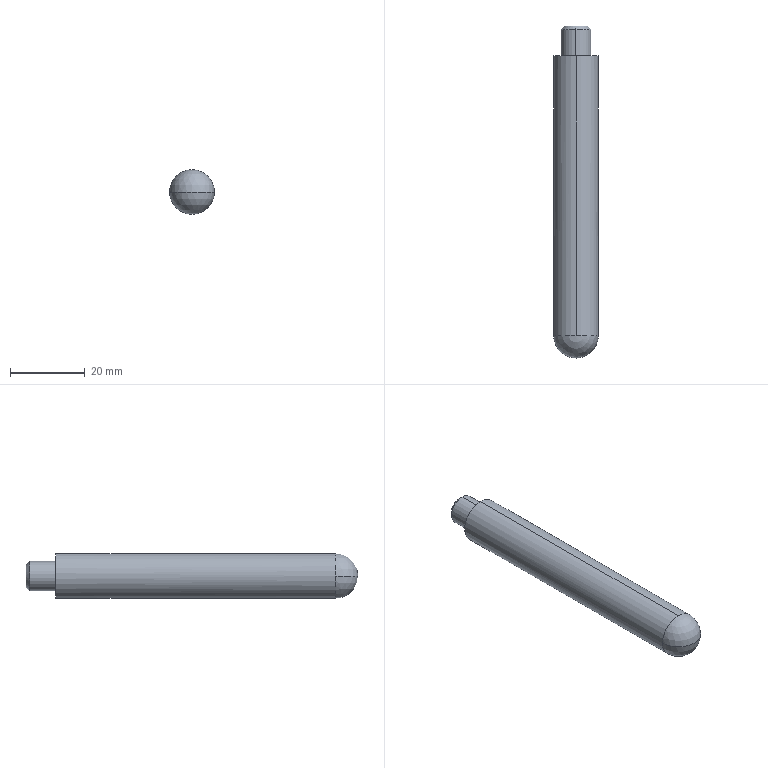Part | SolidWorks | features Chamfer 1, Revolution 1 | 1 solid | 10 faces | box 12 x 89 x 12 mm | volume 9325 mm3 | cylinder 4 | cone 2 | sphere 2 | plane 2 | commonest cylinder face diameters 8 x2 12 x2
STEP:
#1=CARTESIAN_POINT('',(0.,90.,3.));
#2=VERTEX_POINT('',#1);
#3=CARTESIAN_POINT('',(0.,90.,-3.));
#4=VERTEX_POINT('',#3);
#5=CARTESIAN_POINT('',(0.,90.,0.));
#6=DIRECTION('',(0.,1.,0.));
#7=DIRECTION('',(0.,0.,-1.));
#8=AXIS2_PLACEMENT_3D('',#5,#6,#7);
#9=CIRCLE('',#8,3.);
#10=EDGE_CURVE('',#2,#4,#9,.T.);
#11=ORIENTED_EDGE('',*,*,#10,.F.);
#12=CARTESIAN_POINT('',(0.,89.,4.));
#13=VERTEX_POINT('',#12);
#14=CARTESIAN_POINT('',(0.,89.,4.));
#15=DIRECTION('',(0.,-0.7071,0.7071));
#16=VECTOR('',#15,1000.);
#17=LINE('',#14,#16);
#18=EDGE_CURVE('',#2,#13,#17,.T.);
#19=ORIENTED_EDGE('',*,*,#18,.T.);
#20=CARTESIAN_POINT('',(0.,89.,-4.));
#21=VERTEX_POINT('',#20);
#22=CARTESIAN_POINT('',(0.,89.,0.));
#23=DIRECTION('',(0.,-1.,0.));
#24=DIRECTION('',(0.,0.,-1.));
#25=AXIS2_PLACEMENT_3D('',#22,#23,#24);
#26=CIRCLE('',#25,4.);
#27=EDGE_CURVE('',#21,#13,#26,.T.);
#28=ORIENTED_EDGE('',*,*,#27,.F.);
#29=CARTESIAN_POINT('',(0.,89.,-4.));
#30=DIRECTION('',(0.,-0.7071,-0.7071));
#31=VECTOR('',#30,1000.);
#32=LINE('',#29,#31);
#33=EDGE_CURVE('',#4,#21,#32,.T.);
#34=ORIENTED_EDGE('',*,*,#33,.F.);
#35=EDGE_LOOP('',(#11,#19,#28,#34));
#36=FACE_OUTER_BOUND('',#35,.T.);
#37=CARTESIAN_POINT('',(0.,89.,0.));
#38=DIRECTION('',(0.,-1.,0.));
#39=DIRECTION('',(0.,0.,-1.));
#40=AXIS2_PLACEMENT_3D('',#37,#38,#39);
#41=CONICAL_SURFACE('',#40,4.,0.7854);
#42=ADVANCED_FACE('',(#36),#41,.T.);
#43=CARTESIAN_POINT('',(0.,7.,-6.));
#44=VERTEX_POINT('',#43);
#45=CARTESIAN_POINT('',(6.,7.,0.));
#46=VERTEX_POINT('',#45);
#47=CARTESIAN_POINT('',(0.,7.,0.));
#48=DIRECTION('',(0.,-1.,0.));
#49=DIRECTION('',(0.,0.,-1.));
#50=AXIS2_PLACEMENT_3D('',#47,#48,#49);
#51=CIRCLE('',#50,6.);
#52=EDGE_CURVE('',#44,#46,#51,.T.);
#53=ORIENTED_EDGE('',*,*,#52,.T.);
#54=CARTESIAN_POINT('',(0.,1.,0.));
#55=VERTEX_POINT('',#54);
#56=CARTESIAN_POINT('',(0.,7.,0.));
#57=DIRECTION('',(0.,0.,-1.));
#58=DIRECTION('',(-1.,0.,0.));
#59=AXIS2_PLACEMENT_3D('',#56,#57,#58);
#60=CIRCLE('',#59,6.);
#61=EDGE_CURVE('',#46,#55,#60,.T.);
#62=ORIENTED_EDGE('',*,*,#61,.T.);
#63=CARTESIAN_POINT('',(-6.,7.,0.));
#64=VERTEX_POINT('',#63);
#65=CARTESIAN_POINT('',(0.,7.,0.));
#66=DIRECTION('',(0.,0.,1.));
#67=DIRECTION('',(1.,0.,0.));
#68=AXIS2_PLACEMENT_3D('',#65,#66,#67);
#69=CIRCLE('',#68,6.);
#70=EDGE_CURVE('',#64,#55,#69,.T.);
#71=ORIENTED_EDGE('',*,*,#70,.F.);
#72=CARTESIAN_POINT('',(0.,7.,0.));
#73=DIRECTION('',(0.,-1.,0.));
#74=DIRECTION('',(0.,0.,-1.));
#75=AXIS2_PLACEMENT_3D('',#72,#73,#74);
#76=CIRCLE('',#75,6.);
#77=EDGE_CURVE('',#64,#44,#76,.T.);
#78=ORIENTED_EDGE('',*,*,#77,.T.);
#79=EDGE_LOOP('',(#53,#62,#71,#78));
#80=FACE_OUTER_BOUND('',#79,.T.);
#81=CARTESIAN_POINT('',(0.,7.,0.));
#82=DIRECTION('',(0.,0.,-1.));
#83=DIRECTION('',(-1.,0.,0.));
#84=AXIS2_PLACEMENT_3D('',#81,#82,#83);
#85=SPHERICAL_SURFACE('',#84,6.);
#86=ADVANCED_FACE('',(#80),#85,.T.);
#87=CARTESIAN_POINT('',(0.,82.,-6.));
#88=VERTEX_POINT('',#87);
#89=CARTESIAN_POINT('',(0.,82.,6.));
#90=VERTEX_POINT('',#89);
#91=CARTESIAN_POINT('',(0.,82.,0.));
#92=DIRECTION('',(0.,-1.,0.));
#93=DIRECTION('',(0.,0.,-1.));
#94=AXIS2_PLACEMENT_3D('',#91,#92,#93);
#95=CIRCLE('',#94,6.);
#96=EDGE_CURVE('',#88,#90,#95,.T.);
#97=ORIENTED_EDGE('',*,*,#96,.T.);
#98=CARTESIAN_POINT('',(0.,7.,6.));
#99=VERTEX_POINT('',#98);
#100=CARTESIAN_POINT('',(0.,0.,6.));
#101=DIRECTION('',(0.,-1.,0.));
#102=VECTOR('',#101,1000.);
#103=LINE('',#100,#102);
#104=EDGE_CURVE('',#90,#99,#103,.T.);
#105=ORIENTED_EDGE('',*,*,#104,.T.);
#106=CARTESIAN_POINT('',(0.,7.,0.));
#107=DIRECTION('',(0.,-1.,0.));
#108=DIRECTION('',(0.,0.,-1.));
#109=AXIS2_PLACEMENT_3D('',#106,#107,#108);
#110=CIRCLE('',#109,6.);
#111=EDGE_CURVE('',#46,#99,#110,.T.);
#112=ORIENTED_EDGE('',*,*,#111,.F.);
#113=ORIENTED_EDGE('',*,*,#52,.F.);
#114=CARTESIAN_POINT('',(0.,0.,-6.));
#115=DIRECTION('',(0.,-1.,0.));
#116=VECTOR('',#115,1000.);
#117=LINE('',#114,#116);
#118=EDGE_CURVE('',#88,#44,#117,.T.);
#119=ORIENTED_EDGE('',*,*,#118,.F.);
#120=EDGE_LOOP('',(#97,#105,#112,#113,#119));
#121=FACE_OUTER_BOUND('',#120,.T.);
#122=CARTESIAN_POINT('',(0.,0.,0.));
#123=DIRECTION('',(0.,-1.,0.));
#124=DIRECTION('',(0.,0.,-1.));
#125=AXIS2_PLACEMENT_3D('',#122,#123,#124);
#126=CYLINDRICAL_SURFACE('',#125,6.);
#127=ADVANCED_FACE('',(#121),#126,.T.);
#128=ORIENTED_EDGE('',*,*,#27,.T.);
#129=CARTESIAN_POINT('',(0.,82.,4.));
#130=VERTEX_POINT('',#129);
#131=CARTESIAN_POINT('',(0.,0.,4.));
#132=DIRECTION('',(0.,-1.,0.));
#133=VECTOR('',#132,1000.);
#134=LINE('',#131,#133);
#135=EDGE_CURVE('',#13,#130,#134,.T.);
#136=ORIENTED_EDGE('',*,*,#135,.T.);
#137=CARTESIAN_POINT('',(0.,82.,-4.));
#138=VERTEX_POINT('',#137);
#139=CARTESIAN_POINT('',(0.,82.,0.));
#140=DIRECTION('',(0.,-1.,0.));
#141=DIRECTION('',(0.,0.,-1.));
#142=AXIS2_PLACEMENT_3D('',#139,#140,#141);
#143=CIRCLE('',#142,4.);
#144=EDGE_CURVE('',#138,#130,#143,.T.);
#145=ORIENTED_EDGE('',*,*,#144,.F.);
#146=CARTESIAN_POINT('',(0.,0.,-4.));
#147=DIRECTION('',(0.,-1.,0.));
#148=VECTOR('',#147,1000.);
#149=LINE('',#146,#148);
#150=EDGE_CURVE('',#21,#138,#149,.T.);
#151=ORIENTED_EDGE('',*,*,#150,.F.);
#152=EDGE_LOOP('',(#128,#136,#145,#151));
#153=FACE_OUTER_BOUND('',#152,.T.);
#154=CARTESIAN_POINT('',(0.,0.,0.));
#155=DIRECTION('',(0.,-1.,0.));
#156=DIRECTION('',(0.,0.,-1.));
#157=AXIS2_PLACEMENT_3D('',#154,#155,#156);
#158=CYLINDRICAL_SURFACE('',#157,4.);
#159=ADVANCED_FACE('',(#153),#158,.T.);
#160=CARTESIAN_POINT('',(0.,90.,0.));
#161=DIRECTION('',(0.,1.,0.));
#162=DIRECTION('',(0.,0.,-1.));
#163=AXIS2_PLACEMENT_3D('',#160,#161,#162);
#164=CIRCLE('',#163,3.);
#165=EDGE_CURVE('',#4,#2,#164,.T.);
#166=ORIENTED_EDGE('',*,*,#165,.T.);
#167=ORIENTED_EDGE('',*,*,#10,.T.);
#168=EDGE_LOOP('',(#166,#167));
#169=FACE_OUTER_BOUND('',#168,.T.);
#170=CARTESIAN_POINT('',(0.,90.,0.));
#171=DIRECTION('',(0.,-1.,0.));
#172=DIRECTION('',(0.,0.,-1.));
#173=AXIS2_PLACEMENT_3D('',#170,#171,#172);
#174=PLANE('',#173);
#175=ADVANCED_FACE('',(#169),#174,.F.);
#176=ORIENTED_EDGE('',*,*,#135,.F.);
#177=CARTESIAN_POINT('',(0.,89.,0.));
#178=DIRECTION('',(0.,-1.,0.));
#179=DIRECTION('',(0.,0.,-1.));
#180=AXIS2_PLACEMENT_3D('',#177,#178,#179);
#181=CIRCLE('',#180,4.);
#182=EDGE_CURVE('',#13,#21,#181,.T.);
#183=ORIENTED_EDGE('',*,*,#182,.T.);
#184=ORIENTED_EDGE('',*,*,#150,.T.);
#185=CARTESIAN_POINT('',(0.,82.,0.));
#186=DIRECTION('',(0.,-1.,0.));
#187=DIRECTION('',(0.,0.,-1.));
#188=AXIS2_PLACEMENT_3D('',#185,#186,#187);
#189=CIRCLE('',#188,4.);
#190=EDGE_CURVE('',#130,#138,#189,.T.);
#191=ORIENTED_EDGE('',*,*,#190,.F.);
#192=EDGE_LOOP('',(#176,#183,#184,#191));
#193=FACE_OUTER_BOUND('',#192,.T.);
#194=CARTESIAN_POINT('',(0.,0.,0.));
#195=DIRECTION('',(0.,-1.,0.));
#196=DIRECTION('',(0.,0.,-1.));
#197=AXIS2_PLACEMENT_3D('',#194,#195,#196);
#198=CYLINDRICAL_SURFACE('',#197,4.);
#199=ADVANCED_FACE('',(#193),#198,.T.);
#200=ORIENTED_EDGE('',*,*,#96,.F.);
#201=CARTESIAN_POINT('',(0.,82.,0.));
#202=DIRECTION('',(0.,-1.,0.));
#203=DIRECTION('',(0.,0.,-1.));
#204=AXIS2_PLACEMENT_3D('',#201,#202,#203);
#205=CIRCLE('',#204,6.);
#206=EDGE_CURVE('',#90,#88,#205,.T.);
#207=ORIENTED_EDGE('',*,*,#206,.F.);
#208=EDGE_LOOP('',(#200,#207));
#209=FACE_OUTER_BOUND('',#208,.T.);
#210=ORIENTED_EDGE('',*,*,#144,.T.);
#211=ORIENTED_EDGE('',*,*,#190,.T.);
#212=EDGE_LOOP('',(#210,#211));
#213=FACE_BOUND('',#212,.T.);
#214=CARTESIAN_POINT('',(-4.,82.,0.));
#215=DIRECTION('',(0.,-1.,0.));
#216=DIRECTION('',(0.,0.,-1.));
#217=AXIS2_PLACEMENT_3D('',#214,#215,#216);
#218=PLANE('',#217);
#219=ADVANCED_FACE('',(#209,#213),#218,.F.);
#220=ORIENTED_EDGE('',*,*,#104,.F.);
#221=ORIENTED_EDGE('',*,*,#206,.T.);
#222=ORIENTED_EDGE('',*,*,#118,.T.);
#223=ORIENTED_EDGE('',*,*,#77,.F.);
#224=CARTESIAN_POINT('',(0.,7.,0.));
#225=DIRECTION('',(0.,-1.,0.));
#226=DIRECTION('',(0.,0.,-1.));
#227=AXIS2_PLACEMENT_3D('',#224,#225,#226);
#228=CIRCLE('',#227,6.);
#229=EDGE_CURVE('',#99,#64,#228,.T.);
#230=ORIENTED_EDGE('',*,*,#229,.F.);
#231=EDGE_LOOP('',(#220,#221,#222,#223,#230));
#232=FACE_OUTER_BOUND('',#231,.T.);
#233=CARTESIAN_POINT('',(0.,0.,0.));
#234=DIRECTION('',(0.,-1.,0.));
#235=DIRECTION('',(0.,0.,-1.));
#236=AXIS2_PLACEMENT_3D('',#233,#234,#235);
#237=CYLINDRICAL_SURFACE('',#236,6.);
#238=ADVANCED_FACE('',(#232),#237,.T.);
#239=ORIENTED_EDGE('',*,*,#61,.F.);
#240=ORIENTED_EDGE('',*,*,#111,.T.);
#241=ORIENTED_EDGE('',*,*,#229,.T.);
#242=ORIENTED_EDGE('',*,*,#70,.T.);
#243=EDGE_LOOP('',(#239,#240,#241,#242));
#244=FACE_OUTER_BOUND('',#243,.T.);
#245=CARTESIAN_POINT('',(0.,7.,0.));
#246=DIRECTION('',(0.,0.,-1.));
#247=DIRECTION('',(-1.,0.,0.));
#248=AXIS2_PLACEMENT_3D('',#245,#246,#247);
#249=SPHERICAL_SURFACE('',#248,6.);
#250=ADVANCED_FACE('',(#244),#249,.T.);
#251=ORIENTED_EDGE('',*,*,#18,.F.);
#252=ORIENTED_EDGE('',*,*,#165,.F.);
#253=ORIENTED_EDGE('',*,*,#33,.T.);
#254=ORIENTED_EDGE('',*,*,#182,.F.);
#255=EDGE_LOOP('',(#251,#252,#253,#254));
#256=FACE_OUTER_BOUND('',#255,.T.);
#257=CARTESIAN_POINT('',(0.,89.,0.));
#258=DIRECTION('',(0.,-1.,0.));
#259=DIRECTION('',(0.,0.,-1.));
#260=AXIS2_PLACEMENT_3D('',#257,#258,#259);
#261=CONICAL_SURFACE('',#260,4.,0.7854);
#262=ADVANCED_FACE('',(#256),#261,.T.);
#263=CLOSED_SHELL('',(#42,#86,#127,#159,#175,#199,#219,#238,#250,#262));
#264=MANIFOLD_SOLID_BREP('',#263);
#265=CARTESIAN_POINT('',(0.,0.,0.));
#266=DIRECTION('',(0.,0.,1.));
#267=DIRECTION('',(1.,0.,0.));
#268=AXIS2_PLACEMENT_3D('',#265,#266,#267);
#269=(LENGTH_UNIT()NAMED_UNIT(*)SI_UNIT(.MILLI.,.METRE.));
#270=UNCERTAINTY_MEASURE_WITH_UNIT(LENGTH_MEASURE(0.00001),#269,'','');
#271=(NAMED_UNIT(*)PLANE_ANGLE_UNIT()SI_UNIT($,.RADIAN.));
#272=(NAMED_UNIT(*)SI_UNIT($,.STERADIAN.)SOLID_ANGLE_UNIT());
#273=(GEOMETRIC_REPRESENTATION_CONTEXT(3)GLOBAL_UNCERTAINTY_ASSIGNED_CONTEXT((#270))GLOBAL_UNIT_ASSIGNED_CONTEXT((#269,#271,#272))REPRESENTATION_CONTEXT('',''));
#274=ADVANCED_BREP_SHAPE_REPRESENTATION('',(#264,#268),#273);